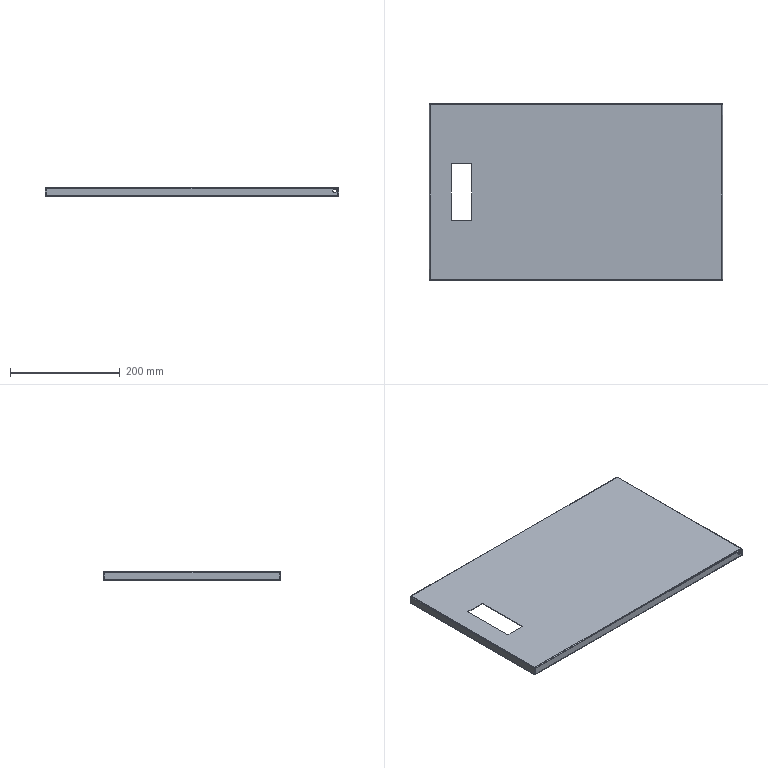Part | STEP file | 1 solid | 94 faces | box 533 x 321 x 16 mm | volume 246500 mm3 | plane 62 | cylinder 20 | spline 12 | commonest cylinder face diameters 1 x8 3.4 x8 6.5 x4